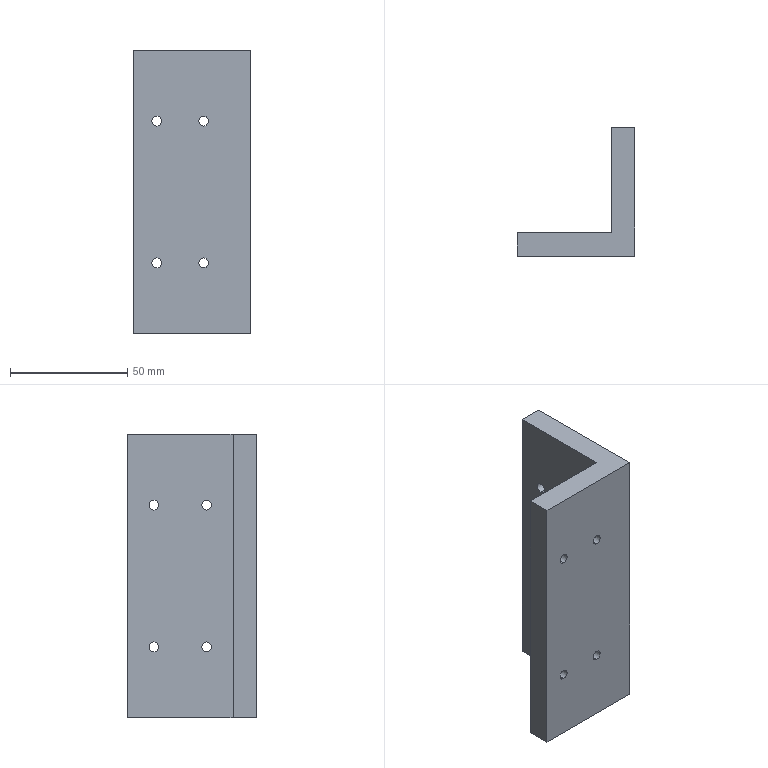Part | SolidWorks | features Cut 1, Extrusion 1, ICE 1 | 1 solid | 24 faces | box 50 x 55 x 121 mm | volume 113842 mm3 | cylinder 16 | plane 8 | commonest cylinder face diameters 4.2 x16
STEP:
#1=CARTESIAN_POINT('',(10.,-9.24,32.35));
#2=VERTEX_POINT('',#1);
#3=CARTESIAN_POINT('',(10.,-9.24,28.15));
#4=VERTEX_POINT('',#3);
#5=CARTESIAN_POINT('',(10.,-9.24,30.25));
#6=DIRECTION('',(1.,0.,0.));
#7=DIRECTION('',(0.,-1.,0.));
#8=AXIS2_PLACEMENT_3D('',#5,#6,#7);
#9=CIRCLE('',#8,2.1);
#10=EDGE_CURVE('',#2,#4,#9,.T.);
#11=ORIENTED_EDGE('',*,*,#10,.T.);
#12=CARTESIAN_POINT('',(0.,-9.24,28.15));
#13=VERTEX_POINT('',#12);
#14=CARTESIAN_POINT('',(15.94,-9.24,28.15));
#15=DIRECTION('',(-1.,0.,0.));
#16=VECTOR('',#15,1000.);
#17=LINE('',#14,#16);
#18=EDGE_CURVE('',#4,#13,#17,.T.);
#19=ORIENTED_EDGE('',*,*,#18,.T.);
#20=CARTESIAN_POINT('',(0.,-9.24,32.35));
#21=VERTEX_POINT('',#20);
#22=CARTESIAN_POINT('',(0.,-9.24,30.25));
#23=DIRECTION('',(-1.,0.,0.));
#24=DIRECTION('',(0.,0.,1.));
#25=AXIS2_PLACEMENT_3D('',#22,#23,#24);
#26=CIRCLE('',#25,2.1);
#27=EDGE_CURVE('',#13,#21,#26,.T.);
#28=ORIENTED_EDGE('',*,*,#27,.T.);
#29=CARTESIAN_POINT('',(15.94,-9.24,32.35));
#30=DIRECTION('',(-1.,0.,0.));
#31=VECTOR('',#30,1000.);
#32=LINE('',#29,#31);
#33=EDGE_CURVE('',#2,#21,#32,.T.);
#34=ORIENTED_EDGE('',*,*,#33,.F.);
#35=EDGE_LOOP('',(#11,#19,#28,#34));
#36=FACE_OUTER_BOUND('',#35,.T.);
#37=CARTESIAN_POINT('',(15.94,-9.24,30.25));
#38=DIRECTION('',(-1.,0.,0.));
#39=DIRECTION('',(0.,0.,1.));
#40=AXIS2_PLACEMENT_3D('',#37,#38,#39);
#41=CYLINDRICAL_SURFACE('',#40,2.1);
#42=ADVANCED_FACE('',(#36),#41,.F.);
#43=CARTESIAN_POINT('',(10.,13.26,92.85));
#44=VERTEX_POINT('',#43);
#45=CARTESIAN_POINT('',(10.,13.26,88.65));
#46=VERTEX_POINT('',#45);
#47=CARTESIAN_POINT('',(10.,13.26,90.75));
#48=DIRECTION('',(1.,0.,0.));
#49=DIRECTION('',(0.,-1.,0.));
#50=AXIS2_PLACEMENT_3D('',#47,#48,#49);
#51=CIRCLE('',#50,2.1);
#52=EDGE_CURVE('',#44,#46,#51,.T.);
#53=ORIENTED_EDGE('',*,*,#52,.T.);
#54=CARTESIAN_POINT('',(0.,13.26,88.65));
#55=VERTEX_POINT('',#54);
#56=CARTESIAN_POINT('',(15.94,13.26,88.65));
#57=DIRECTION('',(-1.,0.,0.));
#58=VECTOR('',#57,1000.);
#59=LINE('',#56,#58);
#60=EDGE_CURVE('',#46,#55,#59,.T.);
#61=ORIENTED_EDGE('',*,*,#60,.T.);
#62=CARTESIAN_POINT('',(0.,13.26,92.85));
#63=VERTEX_POINT('',#62);
#64=CARTESIAN_POINT('',(0.,13.26,90.75));
#65=DIRECTION('',(-1.,0.,0.));
#66=DIRECTION('',(0.,0.,1.));
#67=AXIS2_PLACEMENT_3D('',#64,#65,#66);
#68=CIRCLE('',#67,2.1);
#69=EDGE_CURVE('',#55,#63,#68,.T.);
#70=ORIENTED_EDGE('',*,*,#69,.T.);
#71=CARTESIAN_POINT('',(15.94,13.26,92.85));
#72=DIRECTION('',(-1.,0.,0.));
#73=VECTOR('',#72,1000.);
#74=LINE('',#71,#73);
#75=EDGE_CURVE('',#44,#63,#74,.T.);
#76=ORIENTED_EDGE('',*,*,#75,.F.);
#77=EDGE_LOOP('',(#53,#61,#70,#76));
#78=FACE_OUTER_BOUND('',#77,.T.);
#79=CARTESIAN_POINT('',(15.94,13.26,90.75));
#80=DIRECTION('',(-1.,0.,0.));
#81=DIRECTION('',(0.,0.,1.));
#82=AXIS2_PLACEMENT_3D('',#79,#80,#81);
#83=CYLINDRICAL_SURFACE('',#82,2.1);
#84=ADVANCED_FACE('',(#78),#83,.F.);
#85=CARTESIAN_POINT('',(10.,-9.24,92.85));
#86=VERTEX_POINT('',#85);
#87=CARTESIAN_POINT('',(10.,-9.24,88.65));
#88=VERTEX_POINT('',#87);
#89=CARTESIAN_POINT('',(10.,-9.24,90.75));
#90=DIRECTION('',(1.,0.,0.));
#91=DIRECTION('',(0.,-1.,0.));
#92=AXIS2_PLACEMENT_3D('',#89,#90,#91);
#93=CIRCLE('',#92,2.1);
#94=EDGE_CURVE('',#86,#88,#93,.T.);
#95=ORIENTED_EDGE('',*,*,#94,.T.);
#96=CARTESIAN_POINT('',(0.,-9.24,88.65));
#97=VERTEX_POINT('',#96);
#98=CARTESIAN_POINT('',(15.94,-9.24,88.65));
#99=DIRECTION('',(-1.,0.,0.));
#100=VECTOR('',#99,1000.);
#101=LINE('',#98,#100);
#102=EDGE_CURVE('',#88,#97,#101,.T.);
#103=ORIENTED_EDGE('',*,*,#102,.T.);
#104=CARTESIAN_POINT('',(0.,-9.24,92.85));
#105=VERTEX_POINT('',#104);
#106=CARTESIAN_POINT('',(0.,-9.24,90.75));
#107=DIRECTION('',(-1.,0.,0.));
#108=DIRECTION('',(0.,0.,1.));
#109=AXIS2_PLACEMENT_3D('',#106,#107,#108);
#110=CIRCLE('',#109,2.1);
#111=EDGE_CURVE('',#97,#105,#110,.T.);
#112=ORIENTED_EDGE('',*,*,#111,.T.);
#113=CARTESIAN_POINT('',(15.94,-9.24,92.85));
#114=DIRECTION('',(-1.,0.,0.));
#115=VECTOR('',#114,1000.);
#116=LINE('',#113,#115);
#117=EDGE_CURVE('',#86,#105,#116,.T.);
#118=ORIENTED_EDGE('',*,*,#117,.F.);
#119=EDGE_LOOP('',(#95,#103,#112,#118));
#120=FACE_OUTER_BOUND('',#119,.T.);
#121=CARTESIAN_POINT('',(15.94,-9.24,90.75));
#122=DIRECTION('',(-1.,0.,0.));
#123=DIRECTION('',(0.,0.,1.));
#124=AXIS2_PLACEMENT_3D('',#121,#122,#123);
#125=CYLINDRICAL_SURFACE('',#124,2.1);
#126=ADVANCED_FACE('',(#120),#125,.F.);
#127=CARTESIAN_POINT('',(10.,13.26,32.35));
#128=VERTEX_POINT('',#127);
#129=CARTESIAN_POINT('',(10.,13.26,28.15));
#130=VERTEX_POINT('',#129);
#131=CARTESIAN_POINT('',(10.,13.26,30.25));
#132=DIRECTION('',(1.,0.,0.));
#133=DIRECTION('',(0.,-1.,0.));
#134=AXIS2_PLACEMENT_3D('',#131,#132,#133);
#135=CIRCLE('',#134,2.1);
#136=EDGE_CURVE('',#128,#130,#135,.T.);
#137=ORIENTED_EDGE('',*,*,#136,.T.);
#138=CARTESIAN_POINT('',(0.,13.26,28.15));
#139=VERTEX_POINT('',#138);
#140=CARTESIAN_POINT('',(15.94,13.26,28.15));
#141=DIRECTION('',(-1.,0.,0.));
#142=VECTOR('',#141,1000.);
#143=LINE('',#140,#142);
#144=EDGE_CURVE('',#130,#139,#143,.T.);
#145=ORIENTED_EDGE('',*,*,#144,.T.);
#146=CARTESIAN_POINT('',(0.,13.26,32.35));
#147=VERTEX_POINT('',#146);
#148=CARTESIAN_POINT('',(0.,13.26,30.25));
#149=DIRECTION('',(-1.,0.,0.));
#150=DIRECTION('',(0.,0.,1.));
#151=AXIS2_PLACEMENT_3D('',#148,#149,#150);
#152=CIRCLE('',#151,2.1);
#153=EDGE_CURVE('',#139,#147,#152,.T.);
#154=ORIENTED_EDGE('',*,*,#153,.T.);
#155=CARTESIAN_POINT('',(15.94,13.26,32.35));
#156=DIRECTION('',(-1.,0.,0.));
#157=VECTOR('',#156,1000.);
#158=LINE('',#155,#157);
#159=EDGE_CURVE('',#128,#147,#158,.T.);
#160=ORIENTED_EDGE('',*,*,#159,.F.);
#161=EDGE_LOOP('',(#137,#145,#154,#160));
#162=FACE_OUTER_BOUND('',#161,.T.);
#163=CARTESIAN_POINT('',(15.94,13.26,30.25));
#164=DIRECTION('',(-1.,0.,0.));
#165=DIRECTION('',(0.,0.,1.));
#166=AXIS2_PLACEMENT_3D('',#163,#164,#165);
#167=CYLINDRICAL_SURFACE('',#166,2.1);
#168=ADVANCED_FACE('',(#162),#167,.F.);
#169=CARTESIAN_POINT('',(-10.,-30.49,28.15));
#170=VERTEX_POINT('',#169);
#171=CARTESIAN_POINT('',(-10.,-30.49,32.35));
#172=VERTEX_POINT('',#171);
#173=CARTESIAN_POINT('',(-10.,-30.49,30.25));
#174=DIRECTION('',(0.,1.,0.));
#175=DIRECTION('',(-1.,0.,0.));
#176=AXIS2_PLACEMENT_3D('',#173,#174,#175);
#177=CIRCLE('',#176,2.1);
#178=EDGE_CURVE('',#170,#172,#177,.T.);
#179=ORIENTED_EDGE('',*,*,#178,.F.);
#180=CARTESIAN_POINT('',(-10.,-20.49,28.15));
#181=VERTEX_POINT('',#180);
#182=CARTESIAN_POINT('',(-10.,-51.429,28.15));
#183=DIRECTION('',(0.,1.,0.));
#184=VECTOR('',#183,1000.);
#185=LINE('',#182,#184);
#186=EDGE_CURVE('',#170,#181,#185,.T.);
#187=ORIENTED_EDGE('',*,*,#186,.T.);
#188=CARTESIAN_POINT('',(-10.,-20.49,32.35));
#189=VERTEX_POINT('',#188);
#190=CARTESIAN_POINT('',(-10.,-20.49,30.25));
#191=DIRECTION('',(0.,1.,0.));
#192=DIRECTION('',(0.,0.,1.));
#193=AXIS2_PLACEMENT_3D('',#190,#191,#192);
#194=CIRCLE('',#193,2.1);
#195=EDGE_CURVE('',#181,#189,#194,.T.);
#196=ORIENTED_EDGE('',*,*,#195,.T.);
#197=CARTESIAN_POINT('',(-10.,-51.429,32.35));
#198=DIRECTION('',(0.,1.,0.));
#199=VECTOR('',#198,1000.);
#200=LINE('',#197,#199);
#201=EDGE_CURVE('',#172,#189,#200,.T.);
#202=ORIENTED_EDGE('',*,*,#201,.F.);
#203=EDGE_LOOP('',(#179,#187,#196,#202));
#204=FACE_OUTER_BOUND('',#203,.T.);
#205=CARTESIAN_POINT('',(-10.,-51.429,30.25));
#206=DIRECTION('',(0.,1.,0.));
#207=DIRECTION('',(0.,0.,1.));
#208=AXIS2_PLACEMENT_3D('',#205,#206,#207);
#209=CYLINDRICAL_SURFACE('',#208,2.1);
#210=ADVANCED_FACE('',(#204),#209,.F.);
#211=CARTESIAN_POINT('',(-30.,-30.49,28.15));
#212=VERTEX_POINT('',#211);
#213=CARTESIAN_POINT('',(-30.,-30.49,32.35));
#214=VERTEX_POINT('',#213);
#215=CARTESIAN_POINT('',(-30.,-30.49,30.25));
#216=DIRECTION('',(0.,1.,0.));
#217=DIRECTION('',(-1.,0.,0.));
#218=AXIS2_PLACEMENT_3D('',#215,#216,#217);
#219=CIRCLE('',#218,2.1);
#220=EDGE_CURVE('',#212,#214,#219,.T.);
#221=ORIENTED_EDGE('',*,*,#220,.F.);
#222=CARTESIAN_POINT('',(-30.,-20.49,28.15));
#223=VERTEX_POINT('',#222);
#224=CARTESIAN_POINT('',(-30.,-51.429,28.15));
#225=DIRECTION('',(0.,1.,0.));
#226=VECTOR('',#225,1000.);
#227=LINE('',#224,#226);
#228=EDGE_CURVE('',#212,#223,#227,.T.);
#229=ORIENTED_EDGE('',*,*,#228,.T.);
#230=CARTESIAN_POINT('',(-30.,-20.49,32.35));
#231=VERTEX_POINT('',#230);
#232=CARTESIAN_POINT('',(-30.,-20.49,30.25));
#233=DIRECTION('',(0.,1.,0.));
#234=DIRECTION('',(0.,0.,1.));
#235=AXIS2_PLACEMENT_3D('',#232,#233,#234);
#236=CIRCLE('',#235,2.1);
#237=EDGE_CURVE('',#223,#231,#236,.T.);
#238=ORIENTED_EDGE('',*,*,#237,.T.);
#239=CARTESIAN_POINT('',(-30.,-51.429,32.35));
#240=DIRECTION('',(0.,1.,0.));
#241=VECTOR('',#240,1000.);
#242=LINE('',#239,#241);
#243=EDGE_CURVE('',#214,#231,#242,.T.);
#244=ORIENTED_EDGE('',*,*,#243,.F.);
#245=EDGE_LOOP('',(#221,#229,#238,#244));
#246=FACE_OUTER_BOUND('',#245,.T.);
#247=CARTESIAN_POINT('',(-30.,-51.429,30.25));
#248=DIRECTION('',(0.,1.,0.));
#249=DIRECTION('',(0.,0.,1.));
#250=AXIS2_PLACEMENT_3D('',#247,#248,#249);
#251=CYLINDRICAL_SURFACE('',#250,2.1);
#252=ADVANCED_FACE('',(#246),#251,.F.);
#253=CARTESIAN_POINT('',(-30.,-30.49,88.65));
#254=VERTEX_POINT('',#253);
#255=CARTESIAN_POINT('',(-30.,-30.49,92.85));
#256=VERTEX_POINT('',#255);
#257=CARTESIAN_POINT('',(-30.,-30.49,90.75));
#258=DIRECTION('',(0.,1.,0.));
#259=DIRECTION('',(-1.,0.,0.));
#260=AXIS2_PLACEMENT_3D('',#257,#258,#259);
#261=CIRCLE('',#260,2.1);
#262=EDGE_CURVE('',#254,#256,#261,.T.);
#263=ORIENTED_EDGE('',*,*,#262,.F.);
#264=CARTESIAN_POINT('',(-30.,-20.49,88.65));
#265=VERTEX_POINT('',#264);
#266=CARTESIAN_POINT('',(-30.,-51.429,88.65));
#267=DIRECTION('',(0.,1.,0.));
#268=VECTOR('',#267,1000.);
#269=LINE('',#266,#268);
#270=EDGE_CURVE('',#254,#265,#269,.T.);
#271=ORIENTED_EDGE('',*,*,#270,.T.);
#272=CARTESIAN_POINT('',(-30.,-20.49,92.85));
#273=VERTEX_POINT('',#272);
#274=CARTESIAN_POINT('',(-30.,-20.49,90.75));
#275=DIRECTION('',(0.,1.,0.));
#276=DIRECTION('',(0.,0.,1.));
#277=AXIS2_PLACEMENT_3D('',#274,#275,#276);
#278=CIRCLE('',#277,2.1);
#279=EDGE_CURVE('',#265,#273,#278,.T.);
#280=ORIENTED_EDGE('',*,*,#279,.T.);
#281=CARTESIAN_POINT('',(-30.,-51.429,92.85));
#282=DIRECTION('',(0.,1.,0.));
#283=VECTOR('',#282,1000.);
#284=LINE('',#281,#283);
#285=EDGE_CURVE('',#256,#273,#284,.T.);
#286=ORIENTED_EDGE('',*,*,#285,.F.);
#287=EDGE_LOOP('',(#263,#271,#280,#286));
#288=FACE_OUTER_BOUND('',#287,.T.);
#289=CARTESIAN_POINT('',(-30.,-51.429,90.75));
#290=DIRECTION('',(0.,1.,0.));
#291=DIRECTION('',(0.,0.,1.));
#292=AXIS2_PLACEMENT_3D('',#289,#290,#291);
#293=CYLINDRICAL_SURFACE('',#292,2.1);
#294=ADVANCED_FACE('',(#288),#293,.F.);
#295=CARTESIAN_POINT('',(-10.,-30.49,88.65));
#296=VERTEX_POINT('',#295);
#297=CARTESIAN_POINT('',(-10.,-30.49,92.85));
#298=VERTEX_POINT('',#297);
#299=CARTESIAN_POINT('',(-10.,-30.49,90.75));
#300=DIRECTION('',(0.,1.,0.));
#301=DIRECTION('',(-1.,0.,0.));
#302=AXIS2_PLACEMENT_3D('',#299,#300,#301);
#303=CIRCLE('',#302,2.1);
#304=EDGE_CURVE('',#296,#298,#303,.T.);
#305=ORIENTED_EDGE('',*,*,#304,.F.);
#306=CARTESIAN_POINT('',(-10.,-20.49,88.65));
#307=VERTEX_POINT('',#306);
#308=CARTESIAN_POINT('',(-10.,-51.429,88.65));
#309=DIRECTION('',(0.,1.,0.));
#310=VECTOR('',#309,1000.);
#311=LINE('',#308,#310);
#312=EDGE_CURVE('',#296,#307,#311,.T.);
#313=ORIENTED_EDGE('',*,*,#312,.T.);
#314=CARTESIAN_POINT('',(-10.,-20.49,92.85));
#315=VERTEX_POINT('',#314);
#316=CARTESIAN_POINT('',(-10.,-20.49,90.75));
#317=DIRECTION('',(0.,1.,0.));
#318=DIRECTION('',(0.,0.,1.));
#319=AXIS2_PLACEMENT_3D('',#316,#317,#318);
#320=CIRCLE('',#319,2.1);
#321=EDGE_CURVE('',#307,#315,#320,.T.);
#322=ORIENTED_EDGE('',*,*,#321,.T.);
#323=CARTESIAN_POINT('',(-10.,-51.429,92.85));
#324=DIRECTION('',(0.,1.,0.));
#325=VECTOR('',#324,1000.);
#326=LINE('',#323,#325);
#327=EDGE_CURVE('',#298,#315,#326,.T.);
#328=ORIENTED_EDGE('',*,*,#327,.F.);
#329=EDGE_LOOP('',(#305,#313,#322,#328));
#330=FACE_OUTER_BOUND('',#329,.T.);
#331=CARTESIAN_POINT('',(-10.,-51.429,90.75));
#332=DIRECTION('',(0.,1.,0.));
#333=DIRECTION('',(0.,0.,1.));
#334=AXIS2_PLACEMENT_3D('',#331,#332,#333);
#335=CYLINDRICAL_SURFACE('',#334,2.1);
#336=ADVANCED_FACE('',(#330),#335,.F.);
#337=ORIENTED_EDGE('',*,*,#10,.F.);
#338=CARTESIAN_POINT('',(10.,-9.24,30.25));
#339=DIRECTION('',(1.,0.,0.));
#340=DIRECTION('',(0.,-1.,0.));
#341=AXIS2_PLACEMENT_3D('',#338,#339,#340);
#342=CIRCLE('',#341,2.1);
#343=EDGE_CURVE('',#4,#2,#342,.T.);
#344=ORIENTED_EDGE('',*,*,#343,.F.);
#345=EDGE_LOOP('',(#337,#344));
#346=FACE_BOUND('',#345,.T.);
#347=ORIENTED_EDGE('',*,*,#52,.F.);
#348=CARTESIAN_POINT('',(10.,13.26,90.75));
#349=DIRECTION('',(1.,0.,0.));
#350=DIRECTION('',(0.,-1.,0.));
#351=AXIS2_PLACEMENT_3D('',#348,#349,#350);
#352=CIRCLE('',#351,2.1);
#353=EDGE_CURVE('',#46,#44,#352,.T.);
#354=ORIENTED_EDGE('',*,*,#353,.F.);
#355=EDGE_LOOP('',(#347,#354));
#356=FACE_BOUND('',#355,.T.);
#357=ORIENTED_EDGE('',*,*,#94,.F.);
#358=CARTESIAN_POINT('',(10.,-9.24,90.75));
#359=DIRECTION('',(1.,0.,0.));
#360=DIRECTION('',(0.,-1.,0.));
#361=AXIS2_PLACEMENT_3D('',#358,#359,#360);
#362=CIRCLE('',#361,2.1);
#363=EDGE_CURVE('',#88,#86,#362,.T.);
#364=ORIENTED_EDGE('',*,*,#363,.F.);
#365=EDGE_LOOP('',(#357,#364));
#366=FACE_BOUND('',#365,.T.);
#367=ORIENTED_EDGE('',*,*,#136,.F.);
#368=CARTESIAN_POINT('',(10.,13.26,30.25));
#369=DIRECTION('',(1.,0.,0.));
#370=DIRECTION('',(0.,-1.,0.));
#371=AXIS2_PLACEMENT_3D('',#368,#369,#370);
#372=CIRCLE('',#371,2.1);
#373=EDGE_CURVE('',#130,#128,#372,.T.);
#374=ORIENTED_EDGE('',*,*,#373,.F.);
#375=EDGE_LOOP('',(#367,#374));
#376=FACE_BOUND('',#375,.T.);
#377=CARTESIAN_POINT('',(10.,-30.49,0.));
#378=VERTEX_POINT('',#377);
#379=CARTESIAN_POINT('',(10.,24.51,0.));
#380=VERTEX_POINT('',#379);
#381=CARTESIAN_POINT('',(10.,24.51,0.));
#382=DIRECTION('',(0.,1.,0.));
#383=VECTOR('',#382,1000.);
#384=LINE('',#381,#383);
#385=EDGE_CURVE('',#378,#380,#384,.T.);
#386=ORIENTED_EDGE('',*,*,#385,.T.);
#387=CARTESIAN_POINT('',(10.,24.51,121.));
#388=VERTEX_POINT('',#387);
#389=CARTESIAN_POINT('',(10.,24.51,121.));
#390=DIRECTION('',(0.,0.,-1.));
#391=VECTOR('',#390,1000.);
#392=LINE('',#389,#391);
#393=EDGE_CURVE('',#388,#380,#392,.T.);
#394=ORIENTED_EDGE('',*,*,#393,.F.);
#395=CARTESIAN_POINT('',(10.,-30.49,121.));
#396=VERTEX_POINT('',#395);
#397=CARTESIAN_POINT('',(10.,24.51,121.));
#398=DIRECTION('',(0.,1.,0.));
#399=VECTOR('',#398,1000.);
#400=LINE('',#397,#399);
#401=EDGE_CURVE('',#396,#388,#400,.T.);
#402=ORIENTED_EDGE('',*,*,#401,.F.);
#403=CARTESIAN_POINT('',(10.,-30.49,121.));
#404=DIRECTION('',(0.,0.,-1.));
#405=VECTOR('',#404,1000.);
#406=LINE('',#403,#405);
#407=EDGE_CURVE('',#396,#378,#406,.T.);
#408=ORIENTED_EDGE('',*,*,#407,.T.);
#409=EDGE_LOOP('',(#386,#394,#402,#408));
#410=FACE_OUTER_BOUND('',#409,.T.);
#411=CARTESIAN_POINT('',(10.,24.51,121.));
#412=DIRECTION('',(-1.,0.,0.));
#413=DIRECTION('',(0.,-1.,0.));
#414=AXIS2_PLACEMENT_3D('',#411,#412,#413);
#415=PLANE('',#414);
#416=ADVANCED_FACE('',(#346,#356,#366,#376,#410),#415,.F.);
#417=CARTESIAN_POINT('',(0.,24.51,0.));
#418=VERTEX_POINT('',#417);
#419=CARTESIAN_POINT('',(0.,24.51,0.));
#420=DIRECTION('',(-1.,0.,0.));
#421=VECTOR('',#420,1000.);
#422=LINE('',#419,#421);
#423=EDGE_CURVE('',#380,#418,#422,.T.);
#424=ORIENTED_EDGE('',*,*,#423,.T.);
#425=CARTESIAN_POINT('',(0.,24.51,121.));
#426=VERTEX_POINT('',#425);
#427=CARTESIAN_POINT('',(0.,24.51,121.));
#428=DIRECTION('',(0.,0.,-1.));
#429=VECTOR('',#428,1000.);
#430=LINE('',#427,#429);
#431=EDGE_CURVE('',#426,#418,#430,.T.);
#432=ORIENTED_EDGE('',*,*,#431,.F.);
#433=CARTESIAN_POINT('',(0.,24.51,121.));
#434=DIRECTION('',(-1.,0.,0.));
#435=VECTOR('',#434,1000.);
#436=LINE('',#433,#435);
#437=EDGE_CURVE('',#388,#426,#436,.T.);
#438=ORIENTED_EDGE('',*,*,#437,.F.);
#439=ORIENTED_EDGE('',*,*,#393,.T.);
#440=EDGE_LOOP('',(#424,#432,#438,#439));
#441=FACE_OUTER_BOUND('',#440,.T.);
#442=CARTESIAN_POINT('',(0.,24.51,121.));
#443=DIRECTION('',(0.,-1.,0.));
#444=DIRECTION('',(0.,0.,-1.));
#445=AXIS2_PLACEMENT_3D('',#442,#443,#444);
#446=PLANE('',#445);
#447=ADVANCED_FACE('',(#441),#446,.F.);
#448=CARTESIAN_POINT('',(0.,-9.24,30.25));
#449=DIRECTION('',(-1.,0.,0.));
#450=DIRECTION('',(0.,0.,1.));
#451=AXIS2_PLACEMENT_3D('',#448,#449,#450);
#452=CIRCLE('',#451,2.1);
#453=EDGE_CURVE('',#21,#13,#452,.T.);
#454=ORIENTED_EDGE('',*,*,#453,.F.);
#455=ORIENTED_EDGE('',*,*,#27,.F.);
#456=EDGE_LOOP('',(#454,#455));
#457=FACE_BOUND('',#456,.T.);
#458=CARTESIAN_POINT('',(0.,13.26,90.75));
#459=DIRECTION('',(-1.,0.,0.));
#460=DIRECTION('',(0.,0.,1.));
#461=AXIS2_PLACEMENT_3D('',#458,#459,#460);
#462=CIRCLE('',#461,2.1);
#463=EDGE_CURVE('',#63,#55,#462,.T.);
#464=ORIENTED_EDGE('',*,*,#463,.F.);
#465=ORIENTED_EDGE('',*,*,#69,.F.);
#466=EDGE_LOOP('',(#464,#465));
#467=FACE_BOUND('',#466,.T.);
#468=CARTESIAN_POINT('',(0.,-9.24,90.75));
#469=DIRECTION('',(-1.,0.,0.));
#470=DIRECTION('',(0.,0.,1.));
#471=AXIS2_PLACEMENT_3D('',#468,#469,#470);
#472=CIRCLE('',#471,2.1);
#473=EDGE_CURVE('',#105,#97,#472,.T.);
#474=ORIENTED_EDGE('',*,*,#473,.F.);
#475=ORIENTED_EDGE('',*,*,#111,.F.);
#476=EDGE_LOOP('',(#474,#475));
#477=FACE_BOUND('',#476,.T.);
#478=CARTESIAN_POINT('',(0.,13.26,30.25));
#479=DIRECTION('',(-1.,0.,0.));
#480=DIRECTION('',(0.,0.,1.));
#481=AXIS2_PLACEMENT_3D('',#478,#479,#480);
#482=CIRCLE('',#481,2.1);
#483=EDGE_CURVE('',#147,#139,#482,.T.);
#484=ORIENTED_EDGE('',*,*,#483,.F.);
#485=ORIENTED_EDGE('',*,*,#153,.F.);
#486=EDGE_LOOP('',(#484,#485));
#487=FACE_BOUND('',#486,.T.);
#488=CARTESIAN_POINT('',(0.,-20.49,0.));
#489=VERTEX_POINT('',#488);
#490=CARTESIAN_POINT('',(0.,-20.49,0.));
#491=DIRECTION('',(0.,-1.,0.));
#492=VECTOR('',#491,1000.);
#493=LINE('',#490,#492);
#494=EDGE_CURVE('',#418,#489,#493,.T.);
#495=ORIENTED_EDGE('',*,*,#494,.T.);
#496=CARTESIAN_POINT('',(0.,-20.49,121.));
#497=VERTEX_POINT('',#496);
#498=CARTESIAN_POINT('',(0.,-20.49,121.));
#499=DIRECTION('',(0.,0.,-1.));
#500=VECTOR('',#499,1000.);
#501=LINE('',#498,#500);
#502=EDGE_CURVE('',#497,#489,#501,.T.);
#503=ORIENTED_EDGE('',*,*,#502,.F.);
#504=CARTESIAN_POINT('',(0.,-20.49,121.));
#505=DIRECTION('',(0.,-1.,0.));
#506=VECTOR('',#505,1000.);
#507=LINE('',#504,#506);
#508=EDGE_CURVE('',#426,#497,#507,.T.);
#509=ORIENTED_EDGE('',*,*,#508,.F.);
#510=ORIENTED_EDGE('',*,*,#431,.T.);
#511=EDGE_LOOP('',(#495,#503,#509,#510));
#512=FACE_OUTER_BOUND('',#511,.T.);
#513=CARTESIAN_POINT('',(0.,-20.49,121.));
#514=DIRECTION('',(1.,0.,0.));
#515=DIRECTION('',(0.,0.,-1.));
#516=AXIS2_PLACEMENT_3D('',#513,#514,#515);
#517=PLANE('',#516);
#518=ADVANCED_FACE('',(#457,#467,#477,#487,#512),#517,.F.);
#519=CARTESIAN_POINT('',(-10.,-20.49,30.25));
#520=DIRECTION('',(0.,1.,0.));
#521=DIRECTION('',(0.,0.,1.));
#522=AXIS2_PLACEMENT_3D('',#519,#520,#521);
#523=CIRCLE('',#522,2.1);
#524=EDGE_CURVE('',#189,#181,#523,.T.);
#525=ORIENTED_EDGE('',*,*,#524,.F.);
#526=ORIENTED_EDGE('',*,*,#195,.F.);
#527=EDGE_LOOP('',(#525,#526));
#528=FACE_BOUND('',#527,.T.);
#529=CARTESIAN_POINT('',(-30.,-20.49,30.25));
#530=DIRECTION('',(0.,1.,0.));
#531=DIRECTION('',(0.,0.,1.));
#532=AXIS2_PLACEMENT_3D('',#529,#530,#531);
#533=CIRCLE('',#532,2.1);
#534=EDGE_CURVE('',#231,#223,#533,.T.);
#535=ORIENTED_EDGE('',*,*,#534,.F.);
#536=ORIENTED_EDGE('',*,*,#237,.F.);
#537=EDGE_LOOP('',(#535,#536));
#538=FACE_BOUND('',#537,.T.);
#539=CARTESIAN_POINT('',(-30.,-20.49,90.75));
#540=DIRECTION('',(0.,1.,0.));
#541=DIRECTION('',(0.,0.,1.));
#542=AXIS2_PLACEMENT_3D('',#539,#540,#541);
#543=CIRCLE('',#542,2.1);
#544=EDGE_CURVE('',#273,#265,#543,.T.);
#545=ORIENTED_EDGE('',*,*,#544,.F.);
#546=ORIENTED_EDGE('',*,*,#279,.F.);
#547=EDGE_LOOP('',(#545,#546));
#548=FACE_BOUND('',#547,.T.);
#549=CARTESIAN_POINT('',(-10.,-20.49,90.75));
#550=DIRECTION('',(0.,1.,0.));
#551=DIRECTION('',(0.,0.,1.));
#552=AXIS2_PLACEMENT_3D('',#549,#550,#551);
#553=CIRCLE('',#552,2.1);
#554=EDGE_CURVE('',#315,#307,#553,.T.);
#555=ORIENTED_EDGE('',*,*,#554,.F.);
#556=ORIENTED_EDGE('',*,*,#321,.F.);
#557=EDGE_LOOP('',(#555,#556));
#558=FACE_BOUND('',#557,.T.);
#559=CARTESIAN_POINT('',(-40.,-20.49,0.));
#560=VERTEX_POINT('',#559);
#561=CARTESIAN_POINT('',(-40.,-20.49,0.));
#562=DIRECTION('',(-1.,0.,0.));
#563=VECTOR('',#562,1000.);
#564=LINE('',#561,#563);
#565=EDGE_CURVE('',#489,#560,#564,.T.);
#566=ORIENTED_EDGE('',*,*,#565,.T.);
#567=CARTESIAN_POINT('',(-40.,-20.49,121.));
#568=VERTEX_POINT('',#567);
#569=CARTESIAN_POINT('',(-40.,-20.49,121.));
#570=DIRECTION('',(0.,0.,-1.));
#571=VECTOR('',#570,1000.);
#572=LINE('',#569,#571);
#573=EDGE_CURVE('',#568,#560,#572,.T.);
#574=ORIENTED_EDGE('',*,*,#573,.F.);
#575=CARTESIAN_POINT('',(-40.,-20.49,121.));
#576=DIRECTION('',(-1.,0.,0.));
#577=VECTOR('',#576,1000.);
#578=LINE('',#575,#577);
#579=EDGE_CURVE('',#497,#568,#578,.T.);
#580=ORIENTED_EDGE('',*,*,#579,.F.);
#581=ORIENTED_EDGE('',*,*,#502,.T.);
#582=EDGE_LOOP('',(#566,#574,#580,#581));
#583=FACE_OUTER_BOUND('',#582,.T.);
#584=CARTESIAN_POINT('',(-40.,-20.49,121.));
#585=DIRECTION('',(0.,-1.,0.));
#586=DIRECTION('',(0.,0.,-1.));
#587=AXIS2_PLACEMENT_3D('',#584,#585,#586);
#588=PLANE('',#587);
#589=ADVANCED_FACE('',(#528,#538,#548,#558,#583),#588,.F.);
#590=CARTESIAN_POINT('',(-40.,-30.49,0.));
#591=VERTEX_POINT('',#590);
#592=CARTESIAN_POINT('',(-40.,-30.49,0.));
#593=DIRECTION('',(0.,-1.,0.));
#594=VECTOR('',#593,1000.);
#595=LINE('',#592,#594);
#596=EDGE_CURVE('',#560,#591,#595,.T.);
#597=ORIENTED_EDGE('',*,*,#596,.T.);
#598=CARTESIAN_POINT('',(-40.,-30.49,121.));
#599=VERTEX_POINT('',#598);
#600=CARTESIAN_POINT('',(-40.,-30.49,121.));
#601=DIRECTION('',(0.,0.,-1.));
#602=VECTOR('',#601,1000.);
#603=LINE('',#600,#602);
#604=EDGE_CURVE('',#599,#591,#603,.T.);
#605=ORIENTED_EDGE('',*,*,#604,.F.);
#606=CARTESIAN_POINT('',(-40.,-30.49,121.));
#607=DIRECTION('',(0.,-1.,0.));
#608=VECTOR('',#607,1000.);
#609=LINE('',#606,#608);
#610=EDGE_CURVE('',#568,#599,#609,.T.);
#611=ORIENTED_EDGE('',*,*,#610,.F.);
#612=ORIENTED_EDGE('',*,*,#573,.T.);
#613=EDGE_LOOP('',(#597,#605,#611,#612));
#614=FACE_OUTER_BOUND('',#613,.T.);
#615=CARTESIAN_POINT('',(-40.,-30.49,121.));
#616=DIRECTION('',(1.,0.,0.));
#617=DIRECTION('',(0.,0.,-1.));
#618=AXIS2_PLACEMENT_3D('',#615,#616,#617);
#619=PLANE('',#618);
#620=ADVANCED_FACE('',(#614),#619,.F.);
#621=CARTESIAN_POINT('',(-10.,-30.49,30.25));
#622=DIRECTION('',(0.,1.,0.));
#623=DIRECTION('',(-1.,0.,0.));
#624=AXIS2_PLACEMENT_3D('',#621,#622,#623);
#625=CIRCLE('',#624,2.1);
#626=EDGE_CURVE('',#172,#170,#625,.T.);
#627=ORIENTED_EDGE('',*,*,#626,.T.);
#628=ORIENTED_EDGE('',*,*,#178,.T.);
#629=EDGE_LOOP('',(#627,#628));
#630=FACE_BOUND('',#629,.T.);
#631=CARTESIAN_POINT('',(-30.,-30.49,30.25));
#632=DIRECTION('',(0.,1.,0.));
#633=DIRECTION('',(-1.,0.,0.));
#634=AXIS2_PLACEMENT_3D('',#631,#632,#633);
#635=CIRCLE('',#634,2.1);
#636=EDGE_CURVE('',#214,#212,#635,.T.);
#637=ORIENTED_EDGE('',*,*,#636,.T.);
#638=ORIENTED_EDGE('',*,*,#220,.T.);
#639=EDGE_LOOP('',(#637,#638));
#640=FACE_BOUND('',#639,.T.);
#641=CARTESIAN_POINT('',(-30.,-30.49,90.75));
#642=DIRECTION('',(0.,1.,0.));
#643=DIRECTION('',(-1.,0.,0.));
#644=AXIS2_PLACEMENT_3D('',#641,#642,#643);
#645=CIRCLE('',#644,2.1);
#646=EDGE_CURVE('',#256,#254,#645,.T.);
#647=ORIENTED_EDGE('',*,*,#646,.T.);
#648=ORIENTED_EDGE('',*,*,#262,.T.);
#649=EDGE_LOOP('',(#647,#648));
#650=FACE_BOUND('',#649,.T.);
#651=CARTESIAN_POINT('',(-10.,-30.49,90.75));
#652=DIRECTION('',(0.,1.,0.));
#653=DIRECTION('',(-1.,0.,0.));
#654=AXIS2_PLACEMENT_3D('',#651,#652,#653);
#655=CIRCLE('',#654,2.1);
#656=EDGE_CURVE('',#298,#296,#655,.T.);
#657=ORIENTED_EDGE('',*,*,#656,.T.);
#658=ORIENTED_EDGE('',*,*,#304,.T.);
#659=EDGE_LOOP('',(#657,#658));
#660=FACE_BOUND('',#659,.T.);
#661=CARTESIAN_POINT('',(10.,-30.49,0.));
#662=DIRECTION('',(1.,0.,0.));
#663=VECTOR('',#662,1000.);
#664=LINE('',#661,#663);
#665=EDGE_CURVE('',#591,#378,#664,.T.);
#666=ORIENTED_EDGE('',*,*,#665,.T.);
#667=ORIENTED_EDGE('',*,*,#407,.F.);
#668=CARTESIAN_POINT('',(10.,-30.49,121.));
#669=DIRECTION('',(1.,0.,0.));
#670=VECTOR('',#669,1000.);
#671=LINE('',#668,#670);
#672=EDGE_CURVE('',#599,#396,#671,.T.);
#673=ORIENTED_EDGE('',*,*,#672,.F.);
#674=ORIENTED_EDGE('',*,*,#604,.T.);
#675=EDGE_LOOP('',(#666,#667,#673,#674));
#676=FACE_OUTER_BOUND('',#675,.T.);
#677=CARTESIAN_POINT('',(10.,-30.49,121.));
#678=DIRECTION('',(0.,1.,0.));
#679=DIRECTION('',(-1.,0.,0.));
#680=AXIS2_PLACEMENT_3D('',#677,#678,#679);
#681=PLANE('',#680);
#682=ADVANCED_FACE('',(#630,#640,#650,#660,#676),#681,.F.);
#683=ORIENTED_EDGE('',*,*,#401,.T.);
#684=ORIENTED_EDGE('',*,*,#437,.T.);
#685=ORIENTED_EDGE('',*,*,#508,.T.);
#686=ORIENTED_EDGE('',*,*,#579,.T.);
#687=ORIENTED_EDGE('',*,*,#610,.T.);
#688=ORIENTED_EDGE('',*,*,#672,.T.);
#689=EDGE_LOOP('',(#683,#684,#685,#686,#687,#688));
#690=FACE_OUTER_BOUND('',#689,.T.);
#691=CARTESIAN_POINT('',(0.,0.,121.));
#692=DIRECTION('',(0.,0.,-1.));
#693=DIRECTION('',(-1.,0.,0.));
#694=AXIS2_PLACEMENT_3D('',#691,#692,#693);
#695=PLANE('',#694);
#696=ADVANCED_FACE('',(#690),#695,.F.);
#697=ORIENTED_EDGE('',*,*,#385,.F.);
#698=ORIENTED_EDGE('',*,*,#665,.F.);
#699=ORIENTED_EDGE('',*,*,#596,.F.);
#700=ORIENTED_EDGE('',*,*,#565,.F.);
#701=ORIENTED_EDGE('',*,*,#494,.F.);
#702=ORIENTED_EDGE('',*,*,#423,.F.);
#703=EDGE_LOOP('',(#697,#698,#699,#700,#701,#702));
#704=FACE_OUTER_BOUND('',#703,.T.);
#705=CARTESIAN_POINT('',(0.,0.,0.));
#706=DIRECTION('',(0.,0.,-1.));
#707=DIRECTION('',(-1.,0.,0.));
#708=AXIS2_PLACEMENT_3D('',#705,#706,#707);
#709=PLANE('',#708);
#710=ADVANCED_FACE('',(#704),#709,.T.);
#711=ORIENTED_EDGE('',*,*,#312,.F.);
#712=ORIENTED_EDGE('',*,*,#656,.F.);
#713=ORIENTED_EDGE('',*,*,#327,.T.);
#714=ORIENTED_EDGE('',*,*,#554,.T.);
#715=EDGE_LOOP('',(#711,#712,#713,#714));
#716=FACE_OUTER_BOUND('',#715,.T.);
#717=CARTESIAN_POINT('',(-10.,-51.429,90.75));
#718=DIRECTION('',(0.,1.,0.));
#719=DIRECTION('',(0.,0.,1.));
#720=AXIS2_PLACEMENT_3D('',#717,#718,#719);
#721=CYLINDRICAL_SURFACE('',#720,2.1);
#722=ADVANCED_FACE('',(#716),#721,.F.);
#723=ORIENTED_EDGE('',*,*,#270,.F.);
#724=ORIENTED_EDGE('',*,*,#646,.F.);
#725=ORIENTED_EDGE('',*,*,#285,.T.);
#726=ORIENTED_EDGE('',*,*,#544,.T.);
#727=EDGE_LOOP('',(#723,#724,#725,#726));
#728=FACE_OUTER_BOUND('',#727,.T.);
#729=CARTESIAN_POINT('',(-30.,-51.429,90.75));
#730=DIRECTION('',(0.,1.,0.));
#731=DIRECTION('',(0.,0.,1.));
#732=AXIS2_PLACEMENT_3D('',#729,#730,#731);
#733=CYLINDRICAL_SURFACE('',#732,2.1);
#734=ADVANCED_FACE('',(#728),#733,.F.);
#735=ORIENTED_EDGE('',*,*,#228,.F.);
#736=ORIENTED_EDGE('',*,*,#636,.F.);
#737=ORIENTED_EDGE('',*,*,#243,.T.);
#738=ORIENTED_EDGE('',*,*,#534,.T.);
#739=EDGE_LOOP('',(#735,#736,#737,#738));
#740=FACE_OUTER_BOUND('',#739,.T.);
#741=CARTESIAN_POINT('',(-30.,-51.429,30.25));
#742=DIRECTION('',(0.,1.,0.));
#743=DIRECTION('',(0.,0.,1.));
#744=AXIS2_PLACEMENT_3D('',#741,#742,#743);
#745=CYLINDRICAL_SURFACE('',#744,2.1);
#746=ADVANCED_FACE('',(#740),#745,.F.);
#747=ORIENTED_EDGE('',*,*,#186,.F.);
#748=ORIENTED_EDGE('',*,*,#626,.F.);
#749=ORIENTED_EDGE('',*,*,#201,.T.);
#750=ORIENTED_EDGE('',*,*,#524,.T.);
#751=EDGE_LOOP('',(#747,#748,#749,#750));
#752=FACE_OUTER_BOUND('',#751,.T.);
#753=CARTESIAN_POINT('',(-10.,-51.429,30.25));
#754=DIRECTION('',(0.,1.,0.));
#755=DIRECTION('',(0.,0.,1.));
#756=AXIS2_PLACEMENT_3D('',#753,#754,#755);
#757=CYLINDRICAL_SURFACE('',#756,2.1);
#758=ADVANCED_FACE('',(#752),#757,.F.);
#759=ORIENTED_EDGE('',*,*,#144,.F.);
#760=ORIENTED_EDGE('',*,*,#373,.T.);
#761=ORIENTED_EDGE('',*,*,#159,.T.);
#762=ORIENTED_EDGE('',*,*,#483,.T.);
#763=EDGE_LOOP('',(#759,#760,#761,#762));
#764=FACE_OUTER_BOUND('',#763,.T.);
#765=CARTESIAN_POINT('',(15.94,13.26,30.25));
#766=DIRECTION('',(-1.,0.,0.));
#767=DIRECTION('',(0.,0.,1.));
#768=AXIS2_PLACEMENT_3D('',#765,#766,#767);
#769=CYLINDRICAL_SURFACE('',#768,2.1);
#770=ADVANCED_FACE('',(#764),#769,.F.);
#771=ORIENTED_EDGE('',*,*,#102,.F.);
#772=ORIENTED_EDGE('',*,*,#363,.T.);
#773=ORIENTED_EDGE('',*,*,#117,.T.);
#774=ORIENTED_EDGE('',*,*,#473,.T.);
#775=EDGE_LOOP('',(#771,#772,#773,#774));
#776=FACE_OUTER_BOUND('',#775,.T.);
#777=CARTESIAN_POINT('',(15.94,-9.24,90.75));
#778=DIRECTION('',(-1.,0.,0.));
#779=DIRECTION('',(0.,0.,1.));
#780=AXIS2_PLACEMENT_3D('',#777,#778,#779);
#781=CYLINDRICAL_SURFACE('',#780,2.1);
#782=ADVANCED_FACE('',(#776),#781,.F.);
#783=ORIENTED_EDGE('',*,*,#60,.F.);
#784=ORIENTED_EDGE('',*,*,#353,.T.);
#785=ORIENTED_EDGE('',*,*,#75,.T.);
#786=ORIENTED_EDGE('',*,*,#463,.T.);
#787=EDGE_LOOP('',(#783,#784,#785,#786));
#788=FACE_OUTER_BOUND('',#787,.T.);
#789=CARTESIAN_POINT('',(15.94,13.26,90.75));
#790=DIRECTION('',(-1.,0.,0.));
#791=DIRECTION('',(0.,0.,1.));
#792=AXIS2_PLACEMENT_3D('',#789,#790,#791);
#793=CYLINDRICAL_SURFACE('',#792,2.1);
#794=ADVANCED_FACE('',(#788),#793,.F.);
#795=ORIENTED_EDGE('',*,*,#18,.F.);
#796=ORIENTED_EDGE('',*,*,#343,.T.);
#797=ORIENTED_EDGE('',*,*,#33,.T.);
#798=ORIENTED_EDGE('',*,*,#453,.T.);
#799=EDGE_LOOP('',(#795,#796,#797,#798));
#800=FACE_OUTER_BOUND('',#799,.T.);
#801=CARTESIAN_POINT('',(15.94,-9.24,30.25));
#802=DIRECTION('',(-1.,0.,0.));
#803=DIRECTION('',(0.,0.,1.));
#804=AXIS2_PLACEMENT_3D('',#801,#802,#803);
#805=CYLINDRICAL_SURFACE('',#804,2.1);
#806=ADVANCED_FACE('',(#800),#805,.F.);
#807=CLOSED_SHELL('',(#42,#84,#126,#168,#210,#252,#294,#336,#416,#447,#518,#589,#620,#682,#696,#710,#722,#734,#746,#758,#770,#782,#794,#806));
#808=MANIFOLD_SOLID_BREP('',#807);
#809=CARTESIAN_POINT('',(0.,0.,0.));
#810=DIRECTION('',(0.,0.,1.));
#811=DIRECTION('',(1.,0.,0.));
#812=AXIS2_PLACEMENT_3D('',#809,#810,#811);
#813=(LENGTH_UNIT()NAMED_UNIT(*)SI_UNIT(.MILLI.,.METRE.));
#814=UNCERTAINTY_MEASURE_WITH_UNIT(LENGTH_MEASURE(0.00001),#813,'','');
#815=(NAMED_UNIT(*)PLANE_ANGLE_UNIT()SI_UNIT($,.RADIAN.));
#816=(NAMED_UNIT(*)SI_UNIT($,.STERADIAN.)SOLID_ANGLE_UNIT());
#817=(GEOMETRIC_REPRESENTATION_CONTEXT(3)GLOBAL_UNCERTAINTY_ASSIGNED_CONTEXT((#814))GLOBAL_UNIT_ASSIGNED_CONTEXT((#813,#815,#816))REPRESENTATION_CONTEXT('',''));
#818=ADVANCED_BREP_SHAPE_REPRESENTATION('',(#808,#812),#817);